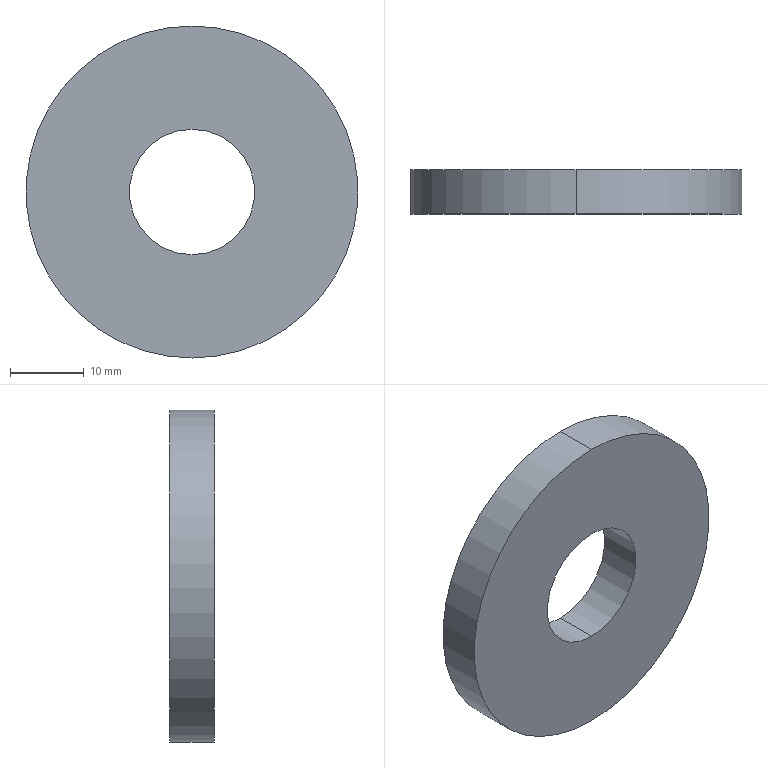Part | SolidWorks | features Extrusion 1 | 1 solid | 6 faces | box 45 x 6 x 45 mm | volume 8181 mm3 | cylinder 4 | plane 2 | commonest cylinder face diameters 17 x2 45 x2
STEP:
#1=CARTESIAN_POINT('',(0.,6.,-8.5));
#2=VERTEX_POINT('',#1);
#3=CARTESIAN_POINT('',(0.,6.,8.5));
#4=VERTEX_POINT('',#3);
#5=CARTESIAN_POINT('',(0.,6.,0.));
#6=DIRECTION('',(0.,1.,0.));
#7=DIRECTION('',(0.,0.,1.));
#8=AXIS2_PLACEMENT_3D('',#5,#6,#7);
#9=CIRCLE('',#8,8.5);
#10=EDGE_CURVE('',#2,#4,#9,.T.);
#11=ORIENTED_EDGE('',*,*,#10,.T.);
#12=CARTESIAN_POINT('',(0.,0.,8.5));
#13=VERTEX_POINT('',#12);
#14=CARTESIAN_POINT('',(0.,6.,8.5));
#15=DIRECTION('',(0.,-1.,0.));
#16=VECTOR('',#15,1000.);
#17=LINE('',#14,#16);
#18=EDGE_CURVE('',#4,#13,#17,.T.);
#19=ORIENTED_EDGE('',*,*,#18,.T.);
#20=CARTESIAN_POINT('',(0.,0.,-8.5));
#21=VERTEX_POINT('',#20);
#22=CARTESIAN_POINT('',(0.,0.,0.));
#23=DIRECTION('',(0.,1.,0.));
#24=DIRECTION('',(0.,0.,1.));
#25=AXIS2_PLACEMENT_3D('',#22,#23,#24);
#26=CIRCLE('',#25,8.5);
#27=EDGE_CURVE('',#21,#13,#26,.T.);
#28=ORIENTED_EDGE('',*,*,#27,.F.);
#29=CARTESIAN_POINT('',(0.,6.,-8.5));
#30=DIRECTION('',(0.,-1.,0.));
#31=VECTOR('',#30,1000.);
#32=LINE('',#29,#31);
#33=EDGE_CURVE('',#2,#21,#32,.T.);
#34=ORIENTED_EDGE('',*,*,#33,.F.);
#35=EDGE_LOOP('',(#11,#19,#28,#34));
#36=FACE_OUTER_BOUND('',#35,.T.);
#37=CARTESIAN_POINT('',(0.,6.,0.));
#38=DIRECTION('',(0.,-1.,0.));
#39=DIRECTION('',(0.,0.,-1.));
#40=AXIS2_PLACEMENT_3D('',#37,#38,#39);
#41=CYLINDRICAL_SURFACE('',#40,8.5);
#42=ADVANCED_FACE('',(#36),#41,.F.);
#43=CARTESIAN_POINT('',(0.,6.,22.5));
#44=VERTEX_POINT('',#43);
#45=CARTESIAN_POINT('',(0.,6.,-22.5));
#46=VERTEX_POINT('',#45);
#47=CARTESIAN_POINT('',(0.,6.,0.));
#48=DIRECTION('',(0.,1.,0.));
#49=DIRECTION('',(0.,0.,1.));
#50=AXIS2_PLACEMENT_3D('',#47,#48,#49);
#51=CIRCLE('',#50,22.5);
#52=EDGE_CURVE('',#44,#46,#51,.T.);
#53=ORIENTED_EDGE('',*,*,#52,.F.);
#54=CARTESIAN_POINT('',(0.,0.,22.5));
#55=VERTEX_POINT('',#54);
#56=CARTESIAN_POINT('',(0.,6.,22.5));
#57=DIRECTION('',(0.,-1.,0.));
#58=VECTOR('',#57,1000.);
#59=LINE('',#56,#58);
#60=EDGE_CURVE('',#44,#55,#59,.T.);
#61=ORIENTED_EDGE('',*,*,#60,.T.);
#62=CARTESIAN_POINT('',(0.,0.,-22.5));
#63=VERTEX_POINT('',#62);
#64=CARTESIAN_POINT('',(0.,0.,0.));
#65=DIRECTION('',(0.,1.,0.));
#66=DIRECTION('',(0.,0.,1.));
#67=AXIS2_PLACEMENT_3D('',#64,#65,#66);
#68=CIRCLE('',#67,22.5);
#69=EDGE_CURVE('',#55,#63,#68,.T.);
#70=ORIENTED_EDGE('',*,*,#69,.T.);
#71=CARTESIAN_POINT('',(0.,6.,-22.5));
#72=DIRECTION('',(0.,-1.,0.));
#73=VECTOR('',#72,1000.);
#74=LINE('',#71,#73);
#75=EDGE_CURVE('',#46,#63,#74,.T.);
#76=ORIENTED_EDGE('',*,*,#75,.F.);
#77=EDGE_LOOP('',(#53,#61,#70,#76));
#78=FACE_OUTER_BOUND('',#77,.T.);
#79=CARTESIAN_POINT('',(0.,6.,0.));
#80=DIRECTION('',(0.,-1.,0.));
#81=DIRECTION('',(0.,0.,-1.));
#82=AXIS2_PLACEMENT_3D('',#79,#80,#81);
#83=CYLINDRICAL_SURFACE('',#82,22.5);
#84=ADVANCED_FACE('',(#78),#83,.T.);
#85=CARTESIAN_POINT('',(0.,6.,0.));
#86=DIRECTION('',(0.,1.,0.));
#87=DIRECTION('',(0.,0.,1.));
#88=AXIS2_PLACEMENT_3D('',#85,#86,#87);
#89=CIRCLE('',#88,22.5);
#90=EDGE_CURVE('',#46,#44,#89,.T.);
#91=ORIENTED_EDGE('',*,*,#90,.T.);
#92=ORIENTED_EDGE('',*,*,#52,.T.);
#93=EDGE_LOOP('',(#91,#92));
#94=FACE_OUTER_BOUND('',#93,.T.);
#95=ORIENTED_EDGE('',*,*,#10,.F.);
#96=CARTESIAN_POINT('',(0.,6.,0.));
#97=DIRECTION('',(0.,1.,0.));
#98=DIRECTION('',(0.,0.,1.));
#99=AXIS2_PLACEMENT_3D('',#96,#97,#98);
#100=CIRCLE('',#99,8.5);
#101=EDGE_CURVE('',#4,#2,#100,.T.);
#102=ORIENTED_EDGE('',*,*,#101,.F.);
#103=EDGE_LOOP('',(#95,#102));
#104=FACE_BOUND('',#103,.T.);
#105=CARTESIAN_POINT('',(0.,6.,0.));
#106=DIRECTION('',(0.,1.,0.));
#107=DIRECTION('',(0.,0.,1.));
#108=AXIS2_PLACEMENT_3D('',#105,#106,#107);
#109=PLANE('',#108);
#110=ADVANCED_FACE('',(#94,#104),#109,.T.);
#111=CARTESIAN_POINT('',(0.,0.,0.));
#112=DIRECTION('',(0.,1.,0.));
#113=DIRECTION('',(0.,0.,1.));
#114=AXIS2_PLACEMENT_3D('',#111,#112,#113);
#115=CIRCLE('',#114,22.5);
#116=EDGE_CURVE('',#63,#55,#115,.T.);
#117=ORIENTED_EDGE('',*,*,#116,.F.);
#118=ORIENTED_EDGE('',*,*,#69,.F.);
#119=EDGE_LOOP('',(#117,#118));
#120=FACE_OUTER_BOUND('',#119,.T.);
#121=ORIENTED_EDGE('',*,*,#27,.T.);
#122=CARTESIAN_POINT('',(0.,0.,0.));
#123=DIRECTION('',(0.,1.,0.));
#124=DIRECTION('',(0.,0.,1.));
#125=AXIS2_PLACEMENT_3D('',#122,#123,#124);
#126=CIRCLE('',#125,8.5);
#127=EDGE_CURVE('',#13,#21,#126,.T.);
#128=ORIENTED_EDGE('',*,*,#127,.T.);
#129=EDGE_LOOP('',(#121,#128));
#130=FACE_BOUND('',#129,.T.);
#131=CARTESIAN_POINT('',(0.,0.,0.));
#132=DIRECTION('',(0.,1.,0.));
#133=DIRECTION('',(0.,0.,1.));
#134=AXIS2_PLACEMENT_3D('',#131,#132,#133);
#135=PLANE('',#134);
#136=ADVANCED_FACE('',(#120,#130),#135,.F.);
#137=ORIENTED_EDGE('',*,*,#60,.F.);
#138=ORIENTED_EDGE('',*,*,#90,.F.);
#139=ORIENTED_EDGE('',*,*,#75,.T.);
#140=ORIENTED_EDGE('',*,*,#116,.T.);
#141=EDGE_LOOP('',(#137,#138,#139,#140));
#142=FACE_OUTER_BOUND('',#141,.T.);
#143=CARTESIAN_POINT('',(0.,6.,0.));
#144=DIRECTION('',(0.,-1.,0.));
#145=DIRECTION('',(0.,0.,-1.));
#146=AXIS2_PLACEMENT_3D('',#143,#144,#145);
#147=CYLINDRICAL_SURFACE('',#146,22.5);
#148=ADVANCED_FACE('',(#142),#147,.T.);
#149=ORIENTED_EDGE('',*,*,#18,.F.);
#150=ORIENTED_EDGE('',*,*,#101,.T.);
#151=ORIENTED_EDGE('',*,*,#33,.T.);
#152=ORIENTED_EDGE('',*,*,#127,.F.);
#153=EDGE_LOOP('',(#149,#150,#151,#152));
#154=FACE_OUTER_BOUND('',#153,.T.);
#155=CARTESIAN_POINT('',(0.,6.,0.));
#156=DIRECTION('',(0.,-1.,0.));
#157=DIRECTION('',(0.,0.,-1.));
#158=AXIS2_PLACEMENT_3D('',#155,#156,#157);
#159=CYLINDRICAL_SURFACE('',#158,8.5);
#160=ADVANCED_FACE('',(#154),#159,.F.);
#161=CLOSED_SHELL('',(#42,#84,#110,#136,#148,#160));
#162=MANIFOLD_SOLID_BREP('',#161);
#163=CARTESIAN_POINT('',(0.,0.,0.));
#164=DIRECTION('',(0.,0.,1.));
#165=DIRECTION('',(1.,0.,0.));
#166=AXIS2_PLACEMENT_3D('',#163,#164,#165);
#167=(LENGTH_UNIT()NAMED_UNIT(*)SI_UNIT(.MILLI.,.METRE.));
#168=UNCERTAINTY_MEASURE_WITH_UNIT(LENGTH_MEASURE(0.00001),#167,'','');
#169=(NAMED_UNIT(*)PLANE_ANGLE_UNIT()SI_UNIT($,.RADIAN.));
#170=(NAMED_UNIT(*)SI_UNIT($,.STERADIAN.)SOLID_ANGLE_UNIT());
#171=(GEOMETRIC_REPRESENTATION_CONTEXT(3)GLOBAL_UNCERTAINTY_ASSIGNED_CONTEXT((#168))GLOBAL_UNIT_ASSIGNED_CONTEXT((#167,#169,#170))REPRESENTATION_CONTEXT('',''));
#172=ADVANCED_BREP_SHAPE_REPRESENTATION('',(#162,#166),#171);